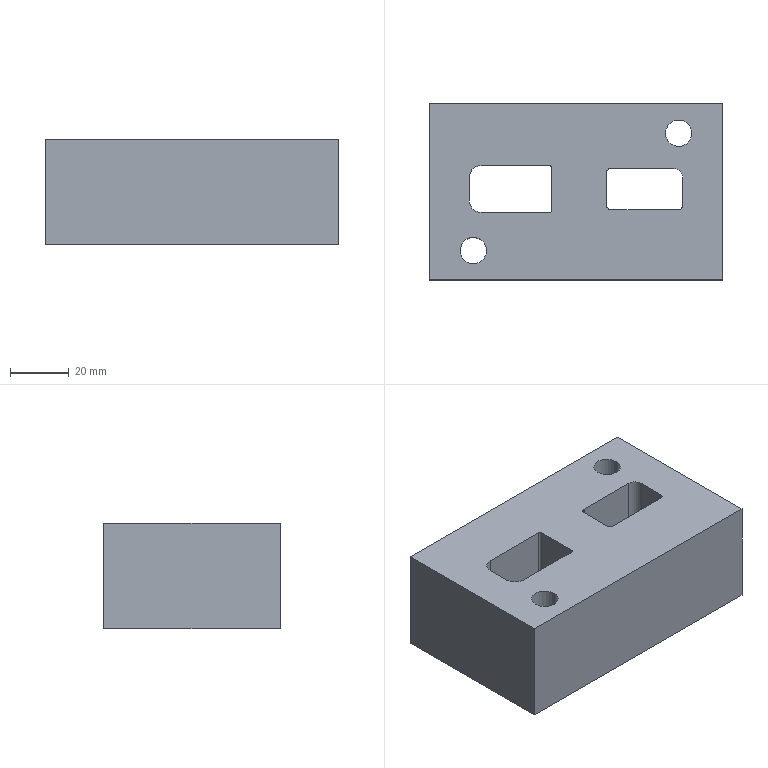Part | 1 solid | 40 faces | box 100 x 60 x 36 mm | volume 178989 mm3 | cylinder 20 | plane 16 | cone 4 | commonest cylinder face diameters 8 x6 9 x4 14 x4 3 x3 1 x2 6 x1